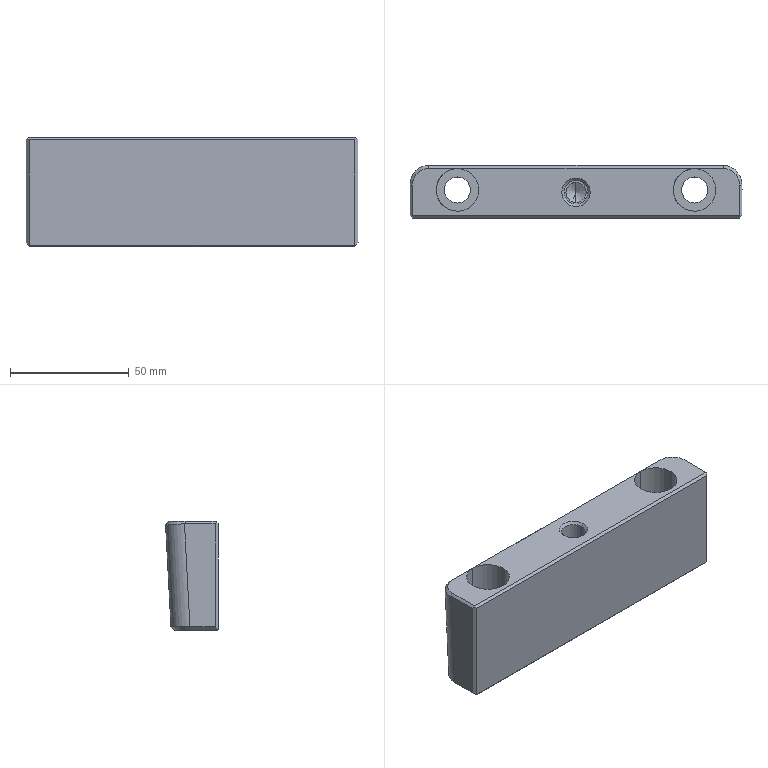Part | Creo | 1 solid | 41 faces | box 140 x 22.308 x 46 mm | volume 119302 mm3 | plane 19 | cylinder 14 | cone 4 | spline 4 | commonest cylinder face diameters 11 x4 18 x4 8.5 x2 10 x2 16 x2
STEP:
#1=CARTESIAN_POINT('',(-4.75,220.995,-77.8));
#2=VERTEX_POINT('',#1);
#3=CARTESIAN_POINT('',(5.25,220.995,-77.8));
#4=VERTEX_POINT('',#3);
#5=CARTESIAN_POINT('',(0.25,220.995,-77.8));
#6=DIRECTION('',(0.,0.,1.));
#7=DIRECTION('',(-1.,0.,0.));
#8=AXIS2_PLACEMENT_3D('',#5,#6,#7);
#9=CIRCLE('',#8,5.);
#10=EDGE_CURVE('',#2,#4,#9,.T.);
#11=ORIENTED_EDGE('',*,*,#10,.F.);
#12=CARTESIAN_POINT('',(0.25,220.995,-77.8));
#13=DIRECTION('',(0.,0.,1.));
#14=DIRECTION('',(1.,0.,0.));
#15=AXIS2_PLACEMENT_3D('',#12,#13,#14);
#16=CIRCLE('',#15,5.);
#17=EDGE_CURVE('',#4,#2,#16,.T.);
#18=ORIENTED_EDGE('',*,*,#17,.F.);
#19=EDGE_LOOP('',(#11,#18));
#20=FACE_OUTER_BOUND('',#19,.F.);
#21=CARTESIAN_POINT('',(-4.,220.995,-77.8));
#22=VERTEX_POINT('',#21);
#23=CARTESIAN_POINT('',(0.25,225.245,-77.8));
#24=VERTEX_POINT('',#23);
#25=CARTESIAN_POINT('',(0.25,220.995,-77.8));
#26=DIRECTION('',(0.,0.,-1.));
#27=DIRECTION('',(-1.,0.,0.));
#28=AXIS2_PLACEMENT_3D('',#25,#26,#27);
#29=CIRCLE('',#28,4.25);
#30=EDGE_CURVE('',#22,#24,#29,.T.);
#31=ORIENTED_EDGE('',*,*,#30,.F.);
#32=CARTESIAN_POINT('',(0.25,216.745,-77.8));
#33=VERTEX_POINT('',#32);
#34=CARTESIAN_POINT('',(0.25,220.995,-77.8));
#35=DIRECTION('',(0.,0.,-1.));
#36=DIRECTION('',(0.000000059,-1.,0.));
#37=AXIS2_PLACEMENT_3D('',#34,#35,#36);
#38=CIRCLE('',#37,4.25);
#39=EDGE_CURVE('',#33,#22,#38,.T.);
#40=ORIENTED_EDGE('',*,*,#39,.F.);
#41=CARTESIAN_POINT('',(0.25,220.995,-77.8));
#42=DIRECTION('',(0.,0.,-1.));
#43=DIRECTION('',(-0.000000059,1.,0.));
#44=AXIS2_PLACEMENT_3D('',#41,#42,#43);
#45=CIRCLE('',#44,4.25);
#46=EDGE_CURVE('',#24,#33,#45,.T.);
#47=ORIENTED_EDGE('',*,*,#46,.F.);
#48=EDGE_LOOP('',(#31,#40,#47));
#49=FACE_BOUND('',#48,.F.);
#50=CARTESIAN_POINT('',(0.25,220.995,-77.8));
#51=DIRECTION('',(0.,0.,-1.));
#52=DIRECTION('',(-1.,0.,0.));
#53=AXIS2_PLACEMENT_3D('',#50,#51,#52);
#54=PLANE('',#53);
#55=ADVANCED_FACE('',(#20,#49),#54,.F.);
#56=ORIENTED_EDGE('',*,*,#39,.T.);
#57=ORIENTED_EDGE('',*,*,#30,.T.);
#58=CARTESIAN_POINT('',(0.25,225.245,-86.8));
#59=VERTEX_POINT('',#58);
#60=CARTESIAN_POINT('',(0.25,225.245,-86.8));
#61=DIRECTION('',(0.,0.,1.));
#62=VECTOR('',#61,9.);
#63=LINE('',#60,#62);
#64=EDGE_CURVE('',#59,#24,#63,.T.);
#65=ORIENTED_EDGE('',*,*,#64,.F.);
#66=CARTESIAN_POINT('',(0.25,216.745,-86.8));
#67=VERTEX_POINT('',#66);
#68=CARTESIAN_POINT('',(0.25,220.995,-86.8));
#69=DIRECTION('',(0.,0.,1.));
#70=DIRECTION('',(-0.000000059,1.,0.));
#71=AXIS2_PLACEMENT_3D('',#68,#69,#70);
#72=CIRCLE('',#71,4.25);
#73=EDGE_CURVE('',#59,#67,#72,.T.);
#74=ORIENTED_EDGE('',*,*,#73,.T.);
#75=CARTESIAN_POINT('',(0.25,216.745,-86.8));
#76=DIRECTION('',(0.,0.,1.));
#77=VECTOR('',#76,9.);
#78=LINE('',#75,#77);
#79=EDGE_CURVE('',#67,#33,#78,.T.);
#80=ORIENTED_EDGE('',*,*,#79,.T.);
#81=EDGE_LOOP('',(#56,#57,#65,#74,#80));
#82=FACE_OUTER_BOUND('',#81,.F.);
#83=CARTESIAN_POINT('',(0.25,220.995,-90.756));
#84=DIRECTION('',(0.,0.,1.));
#85=DIRECTION('',(-0.000000059,1.,0.));
#86=AXIS2_PLACEMENT_3D('',#83,#84,#85);
#87=CYLINDRICAL_SURFACE('',#86,4.25);
#88=ADVANCED_FACE('',(#82),#87,.F.);
#89=ORIENTED_EDGE('',*,*,#46,.T.);
#90=ORIENTED_EDGE('',*,*,#79,.F.);
#91=CARTESIAN_POINT('',(0.25,220.995,-86.8));
#92=DIRECTION('',(0.,0.,1.));
#93=DIRECTION('',(0.000000059,-1.,0.));
#94=AXIS2_PLACEMENT_3D('',#91,#92,#93);
#95=CIRCLE('',#94,4.25);
#96=EDGE_CURVE('',#67,#59,#95,.T.);
#97=ORIENTED_EDGE('',*,*,#96,.T.);
#98=ORIENTED_EDGE('',*,*,#64,.T.);
#99=EDGE_LOOP('',(#89,#90,#97,#98));
#100=FACE_OUTER_BOUND('',#99,.F.);
#101=CARTESIAN_POINT('',(0.25,220.995,-90.756));
#102=DIRECTION('',(0.,0.,1.));
#103=DIRECTION('',(-0.000000059,1.,0.));
#104=AXIS2_PLACEMENT_3D('',#101,#102,#103);
#105=CYLINDRICAL_SURFACE('',#104,4.25);
#106=ADVANCED_FACE('',(#100),#105,.F.);
#107=ORIENTED_EDGE('',*,*,#96,.F.);
#108=CARTESIAN_POINT('',(0.25,220.995,-89.354));
#109=VERTEX_POINT('',#108);
#110=CARTESIAN_POINT('',(0.25,220.995,-89.354));
#111=DIRECTION('',(0.00000005,-0.8572,0.515));
#112=VECTOR('',#111,4.958);
#113=LINE('',#110,#112);
#114=EDGE_CURVE('',#109,#67,#113,.T.);
#115=ORIENTED_EDGE('',*,*,#114,.F.);
#116=CARTESIAN_POINT('',(0.25,220.995,-89.354));
#117=DIRECTION('',(-0.00000005,0.8572,0.515));
#118=VECTOR('',#117,4.958);
#119=LINE('',#116,#118);
#120=EDGE_CURVE('',#109,#59,#119,.T.);
#121=ORIENTED_EDGE('',*,*,#120,.T.);
#122=EDGE_LOOP('',(#107,#115,#121));
#123=FACE_OUTER_BOUND('',#122,.F.);
#124=CARTESIAN_POINT('',(0.25,220.995,-88.03));
#125=DIRECTION('',(0.,0.,1.));
#126=DIRECTION('',(-0.000000059,1.,0.));
#127=AXIS2_PLACEMENT_3D('',#124,#125,#126);
#128=CONICAL_SURFACE('',#127,2.202,59.);
#129=ADVANCED_FACE('',(#123),#128,.F.);
#130=ORIENTED_EDGE('',*,*,#73,.F.);
#131=ORIENTED_EDGE('',*,*,#120,.F.);
#132=ORIENTED_EDGE('',*,*,#114,.T.);
#133=EDGE_LOOP('',(#130,#131,#132));
#134=FACE_OUTER_BOUND('',#133,.F.);
#135=CARTESIAN_POINT('',(0.25,220.995,-88.03));
#136=DIRECTION('',(0.,0.,1.));
#137=DIRECTION('',(-0.000000059,1.,0.));
#138=AXIS2_PLACEMENT_3D('',#135,#136,#137);
#139=CONICAL_SURFACE('',#138,2.202,59.);
#140=ADVANCED_FACE('',(#134),#139,.F.);
#141=CARTESIAN_POINT('',(5.25,220.995,-55.));
#142=VERTEX_POINT('',#141);
#143=CARTESIAN_POINT('',(-4.75,220.995,-55.));
#144=VERTEX_POINT('',#143);
#145=CARTESIAN_POINT('',(0.25,220.995,-55.));
#146=DIRECTION('',(0.,0.,-1.));
#147=DIRECTION('',(1.,0.,0.));
#148=AXIS2_PLACEMENT_3D('',#145,#146,#147);
#149=CIRCLE('',#148,5.);
#150=EDGE_CURVE('',#142,#144,#149,.T.);
#151=ORIENTED_EDGE('',*,*,#150,.T.);
#152=CARTESIAN_POINT('',(-4.75,220.995,-55.));
#153=DIRECTION('',(0.,0.,-1.));
#154=VECTOR('',#153,22.8);
#155=LINE('',#152,#154);
#156=EDGE_CURVE('',#144,#2,#155,.T.);
#157=ORIENTED_EDGE('',*,*,#156,.T.);
#158=ORIENTED_EDGE('',*,*,#10,.T.);
#159=CARTESIAN_POINT('',(5.25,220.995,-55.));
#160=DIRECTION('',(0.,0.,-1.));
#161=VECTOR('',#160,22.8);
#162=LINE('',#159,#161);
#163=EDGE_CURVE('',#142,#4,#162,.T.);
#164=ORIENTED_EDGE('',*,*,#163,.F.);
#165=EDGE_LOOP('',(#151,#157,#158,#164));
#166=FACE_OUTER_BOUND('',#165,.F.);
#167=CARTESIAN_POINT('',(0.25,220.995,-50.3));
#168=DIRECTION('',(0.,0.,-1.));
#169=DIRECTION('',(-1.,0.,0.));
#170=AXIS2_PLACEMENT_3D('',#167,#168,#169);
#171=CYLINDRICAL_SURFACE('',#170,5.);
#172=ADVANCED_FACE('',(#166),#171,.F.);
#173=CARTESIAN_POINT('',(6.25,220.995,-54.));
#174=VERTEX_POINT('',#173);
#175=CARTESIAN_POINT('',(-5.75,220.995,-54.));
#176=VERTEX_POINT('',#175);
#177=CARTESIAN_POINT('',(0.25,220.995,-54.));
#178=DIRECTION('',(0.,0.,-1.));
#179=DIRECTION('',(1.,0.,0.));
#180=AXIS2_PLACEMENT_3D('',#177,#178,#179);
#181=CIRCLE('',#180,6.);
#182=EDGE_CURVE('',#174,#176,#181,.T.);
#183=ORIENTED_EDGE('',*,*,#182,.T.);
#184=CARTESIAN_POINT('',(-4.75,220.995,-55.));
#185=DIRECTION('',(-0.7071,0.,0.7071));
#186=VECTOR('',#185,1.414);
#187=LINE('',#184,#186);
#188=EDGE_CURVE('',#144,#176,#187,.T.);
#189=ORIENTED_EDGE('',*,*,#188,.F.);
#190=ORIENTED_EDGE('',*,*,#150,.F.);
#191=CARTESIAN_POINT('',(5.25,220.995,-55.));
#192=DIRECTION('',(0.7071,0.,0.7071));
#193=VECTOR('',#192,1.414);
#194=LINE('',#191,#193);
#195=EDGE_CURVE('',#142,#174,#194,.T.);
#196=ORIENTED_EDGE('',*,*,#195,.T.);
#197=EDGE_LOOP('',(#183,#189,#190,#196));
#198=FACE_OUTER_BOUND('',#197,.F.);
#199=CARTESIAN_POINT('',(0.25,220.995,-54.5));
#200=DIRECTION('',(0.,0.,1.));
#201=DIRECTION('',(1.,0.,0.));
#202=AXIS2_PLACEMENT_3D('',#199,#200,#201);
#203=CONICAL_SURFACE('',#202,5.5,45.);
#204=ADVANCED_FACE('',(#198),#203,.F.);
#205=CARTESIAN_POINT('',(-68.75,210.995,-54.));
#206=VERTEX_POINT('',#205);
#207=CARTESIAN_POINT('',(-68.75,224.025,-54.));
#208=VERTEX_POINT('',#207);
#209=CARTESIAN_POINT('',(-68.75,210.995,-54.));
#210=DIRECTION('',(0.000008474,1.,0.));
#211=VECTOR('',#210,13.03);
#212=LINE('',#209,#211);
#213=EDGE_CURVE('',#206,#208,#212,.T.);
#214=ORIENTED_EDGE('',*,*,#213,.T.);
#215=CARTESIAN_POINT('',(-61.751,231.036,-54.));
#216=VERTEX_POINT('',#215);
#217=CARTESIAN_POINT('',(-61.745,224.031,-54.));
#218=DIRECTION('',(0.,0.,1.));
#219=DIRECTION('',(-0.001152,1.,0.));
#220=AXIS2_PLACEMENT_3D('',#217,#218,#219);
#221=CIRCLE('',#220,7.005);
#222=EDGE_CURVE('',#216,#208,#221,.T.);
#223=ORIENTED_EDGE('',*,*,#222,.F.);
#224=CARTESIAN_POINT('',(62.253,231.036,-54.));
#225=VERTEX_POINT('',#224);
#226=CARTESIAN_POINT('',(-61.751,231.036,-54.));
#227=DIRECTION('',(1.,0.000000059,0.));
#228=VECTOR('',#227,124.002);
#229=LINE('',#226,#228);
#230=EDGE_CURVE('',#216,#225,#229,.T.);
#231=ORIENTED_EDGE('',*,*,#230,.T.);
#232=CARTESIAN_POINT('',(69.25,224.025,-54.));
#233=VERTEX_POINT('',#232);
#234=CARTESIAN_POINT('',(62.245,224.031,-54.));
#235=DIRECTION('',(0.,0.,1.));
#236=DIRECTION('',(1.,-0.001156,0.));
#237=AXIS2_PLACEMENT_3D('',#234,#235,#236);
#238=CIRCLE('',#237,7.005);
#239=EDGE_CURVE('',#233,#225,#238,.T.);
#240=ORIENTED_EDGE('',*,*,#239,.F.);
#241=CARTESIAN_POINT('',(69.25,210.995,-54.));
#242=VERTEX_POINT('',#241);
#243=CARTESIAN_POINT('',(69.25,224.025,-54.));
#244=DIRECTION('',(0.000004325,-1.,0.000004267));
#245=VECTOR('',#244,13.03);
#246=LINE('',#243,#245);
#247=EDGE_CURVE('',#233,#242,#246,.T.);
#248=ORIENTED_EDGE('',*,*,#247,.T.);
#249=CARTESIAN_POINT('',(69.25,210.995,-54.));
#250=DIRECTION('',(-1.,-0.000000059,0.));
#251=VECTOR('',#250,138.);
#252=LINE('',#249,#251);
#253=EDGE_CURVE('',#242,#206,#252,.T.);
#254=ORIENTED_EDGE('',*,*,#253,.T.);
#255=EDGE_LOOP('',(#214,#223,#231,#240,#248,#254));
#256=FACE_OUTER_BOUND('',#255,.F.);
#257=CARTESIAN_POINT('',(0.25,220.995,-54.));
#258=DIRECTION('',(0.,0.,-1.));
#259=DIRECTION('',(-1.,0.,0.));
#260=AXIS2_PLACEMENT_3D('',#257,#258,#259);
#261=CIRCLE('',#260,6.);
#262=EDGE_CURVE('',#176,#174,#261,.T.);
#263=ORIENTED_EDGE('',*,*,#262,.F.);
#264=ORIENTED_EDGE('',*,*,#182,.F.);
#265=EDGE_LOOP('',(#263,#264));
#266=FACE_BOUND('',#265,.F.);
#267=CARTESIAN_POINT('',(41.25,221.995,-54.));
#268=VERTEX_POINT('',#267);
#269=CARTESIAN_POINT('',(50.25,230.995,-54.));
#270=VERTEX_POINT('',#269);
#271=CARTESIAN_POINT('',(50.25,221.995,-54.));
#272=DIRECTION('',(0.,0.,-1.));
#273=DIRECTION('',(-1.,0.,0.));
#274=AXIS2_PLACEMENT_3D('',#271,#272,#273);
#275=CIRCLE('',#274,9.);
#276=EDGE_CURVE('',#268,#270,#275,.T.);
#277=ORIENTED_EDGE('',*,*,#276,.F.);
#278=CARTESIAN_POINT('',(50.25,212.995,-54.));
#279=VERTEX_POINT('',#278);
#280=CARTESIAN_POINT('',(50.25,221.995,-54.));
#281=DIRECTION('',(0.,0.,-1.));
#282=DIRECTION('',(0.000000059,-1.,0.));
#283=AXIS2_PLACEMENT_3D('',#280,#281,#282);
#284=CIRCLE('',#283,9.);
#285=EDGE_CURVE('',#279,#268,#284,.T.);
#286=ORIENTED_EDGE('',*,*,#285,.F.);
#287=CARTESIAN_POINT('',(50.25,221.995,-54.));
#288=DIRECTION('',(0.,0.,-1.));
#289=DIRECTION('',(-0.000000059,1.,0.));
#290=AXIS2_PLACEMENT_3D('',#287,#288,#289);
#291=CIRCLE('',#290,9.);
#292=EDGE_CURVE('',#270,#279,#291,.T.);
#293=ORIENTED_EDGE('',*,*,#292,.F.);
#294=EDGE_LOOP('',(#277,#286,#293));
#295=FACE_BOUND('',#294,.F.);
#296=CARTESIAN_POINT('',(-58.75,221.995,-54.));
#297=VERTEX_POINT('',#296);
#298=CARTESIAN_POINT('',(-49.75,230.995,-54.));
#299=VERTEX_POINT('',#298);
#300=CARTESIAN_POINT('',(-49.75,221.995,-54.));
#301=DIRECTION('',(0.,0.,-1.));
#302=DIRECTION('',(-1.,0.,0.));
#303=AXIS2_PLACEMENT_3D('',#300,#301,#302);
#304=CIRCLE('',#303,9.);
#305=EDGE_CURVE('',#297,#299,#304,.T.);
#306=ORIENTED_EDGE('',*,*,#305,.F.);
#307=CARTESIAN_POINT('',(-49.75,212.995,-54.));
#308=VERTEX_POINT('',#307);
#309=CARTESIAN_POINT('',(-49.75,221.995,-54.));
#310=DIRECTION('',(0.,0.,-1.));
#311=DIRECTION('',(0.000000059,-1.,0.));
#312=AXIS2_PLACEMENT_3D('',#309,#310,#311);
#313=CIRCLE('',#312,9.);
#314=EDGE_CURVE('',#308,#297,#313,.T.);
#315=ORIENTED_EDGE('',*,*,#314,.F.);
#316=CARTESIAN_POINT('',(-49.75,221.995,-54.));
#317=DIRECTION('',(0.,0.,-1.));
#318=DIRECTION('',(-0.000000059,1.,0.));
#319=AXIS2_PLACEMENT_3D('',#316,#317,#318);
#320=CIRCLE('',#319,9.);
#321=EDGE_CURVE('',#299,#308,#320,.T.);
#322=ORIENTED_EDGE('',*,*,#321,.F.);
#323=EDGE_LOOP('',(#306,#315,#322));
#324=FACE_BOUND('',#323,.F.);
#325=CARTESIAN_POINT('',(0.25,286.495,-54.));
#326=DIRECTION('',(0.,0.,-1.));
#327=DIRECTION('',(-1.,0.,0.));
#328=AXIS2_PLACEMENT_3D('',#325,#326,#327);
#329=PLANE('',#328);
#330=ADVANCED_FACE('',(#256,#266,#295,#324),#329,.F.);
#331=CARTESIAN_POINT('',(-69.75,224.026,-55.));
#332=VERTEX_POINT('',#331);
#333=CARTESIAN_POINT('',(-69.75,211.419,-55.));
#334=VERTEX_POINT('',#333);
#335=CARTESIAN_POINT('',(-69.75,224.026,-55.));
#336=DIRECTION('',(-0.000003827,-1.,0.000003886));
#337=VECTOR('',#336,12.608);
#338=LINE('',#335,#337);
#339=EDGE_CURVE('',#332,#334,#338,.T.);
#340=ORIENTED_EDGE('',*,*,#339,.F.);
#341=CARTESIAN_POINT('',(-69.75,224.026,-55.));
#342=DIRECTION('',(0.7071,-0.0006986,0.7071));
#343=VECTOR('',#342,1.414);
#344=LINE('',#341,#343);
#345=EDGE_CURVE('',#332,#208,#344,.T.);
#346=ORIENTED_EDGE('',*,*,#345,.T.);
#347=ORIENTED_EDGE('',*,*,#213,.F.);
#348=CARTESIAN_POINT('',(-69.038,210.707,-54.288));
#349=VERTEX_POINT('',#348);
#350=CARTESIAN_POINT('',(-69.038,210.707,-54.288));
#351=DIRECTION('',(0.5774,0.5774,0.5774));
#352=VECTOR('',#351,0.4993);
#353=LINE('',#350,#352);
#354=EDGE_CURVE('',#349,#206,#353,.T.);
#355=ORIENTED_EDGE('',*,*,#354,.F.);
#356=CARTESIAN_POINT('',(-69.75,211.419,-55.));
#357=DIRECTION('',(0.5774,-0.5774,0.5774));
#358=VECTOR('',#357,1.233);
#359=LINE('',#356,#358);
#360=EDGE_CURVE('',#334,#349,#359,.T.);
#361=ORIENTED_EDGE('',*,*,#360,.F.);
#362=EDGE_LOOP('',(#340,#346,#347,#355,#361));
#363=FACE_OUTER_BOUND('',#362,.F.);
#364=CARTESIAN_POINT('',(-69.75,209.995,-55.));
#365=DIRECTION('',(0.7071,0.000000042,-0.7071));
#366=DIRECTION('',(-0.000000059,1.,0.));
#367=AXIS2_PLACEMENT_3D('',#364,#365,#366);
#368=PLANE('',#367);
#369=ADVANCED_FACE('',(#363),#368,.F.);
#370=CARTESIAN_POINT('',(-69.75,211.419,-98.419));
#371=VERTEX_POINT('',#370);
#372=CARTESIAN_POINT('',(-69.75,211.419,-55.));
#373=DIRECTION('',(0.,0.,-1.));
#374=VECTOR('',#373,43.419);
#375=LINE('',#372,#374);
#376=EDGE_CURVE('',#334,#371,#375,.T.);
#377=ORIENTED_EDGE('',*,*,#376,.T.);
#378=CARTESIAN_POINT('',(-69.75,222.039,-98.419));
#379=VERTEX_POINT('',#378);
#380=CARTESIAN_POINT('',(-69.75,211.419,-98.419));
#381=DIRECTION('',(-0.000000059,1.,-0.00001364));
#382=VECTOR('',#381,10.62);
#383=LINE('',#380,#382);
#384=EDGE_CURVE('',#371,#379,#383,.T.);
#385=ORIENTED_EDGE('',*,*,#384,.T.);
#386=CARTESIAN_POINT('',(-69.75,224.314,-55.007));
#387=VERTEX_POINT('',#386);
#388=CARTESIAN_POINT('',(-69.75,224.314,-55.007));
#389=DIRECTION('',(-0.000000814,-0.05234,-0.9986));
#390=VECTOR('',#389,43.472);
#391=LINE('',#388,#390);
#392=EDGE_CURVE('',#387,#379,#391,.T.);
#393=ORIENTED_EDGE('',*,*,#392,.F.);
#394=CARTESIAN_POINT('',(-69.75,224.026,-55.));
#395=CARTESIAN_POINT('',(-69.75,224.058,-55.));
#396=CARTESIAN_POINT('',(-69.75,224.122,-55.001));
#397=CARTESIAN_POINT('',(-69.75,224.218,-55.003));
#398=CARTESIAN_POINT('',(-69.75,224.282,-55.006));
#399=B_SPLINE_CURVE_WITH_KNOTS('',3,(#394,#395,#396,#397,#398,#386),.UNSPECIFIED.,.F.,.F.,(4,1,1,4),(0.,0.3333,0.6667,1.),.UNSPECIFIED.);
#400=EDGE_CURVE('',#332,#387,#399,.T.);
#401=ORIENTED_EDGE('',*,*,#400,.F.);
#402=ORIENTED_EDGE('',*,*,#339,.T.);
#403=EDGE_LOOP('',(#377,#385,#393,#401,#402));
#404=FACE_OUTER_BOUND('',#403,.F.);
#405=CARTESIAN_POINT('',(-69.75,209.995,-61.3));
#406=DIRECTION('',(1.,0.000000059,0.));
#407=DIRECTION('',(-0.000000059,1.,0.));
#408=AXIS2_PLACEMENT_3D('',#405,#406,#407);
#409=PLANE('',#408);
#410=ADVANCED_FACE('',(#404),#409,.F.);
#411=CARTESIAN_POINT('',(-68.498,210.167,-99.671));
#412=VERTEX_POINT('',#411);
#413=CARTESIAN_POINT('',(-69.75,211.419,-98.419));
#414=DIRECTION('',(0.5774,-0.5774,-0.5774));
#415=VECTOR('',#414,2.169);
#416=LINE('',#413,#415);
#417=EDGE_CURVE('',#371,#412,#416,.T.);
#418=ORIENTED_EDGE('',*,*,#417,.F.);
#419=ORIENTED_EDGE('',*,*,#376,.F.);
#420=ORIENTED_EDGE('',*,*,#360,.T.);
#421=CARTESIAN_POINT('',(-68.331,210.,-54.995));
#422=VERTEX_POINT('',#421);
#423=CARTESIAN_POINT('',(-69.038,210.707,-54.288));
#424=DIRECTION('',(0.5774,-0.5774,-0.5774));
#425=VECTOR('',#424,1.225);
#426=LINE('',#423,#425);
#427=EDGE_CURVE('',#349,#422,#426,.T.);
#428=ORIENTED_EDGE('',*,*,#427,.T.);
#429=CARTESIAN_POINT('',(-68.331,210.,-99.505));
#430=VERTEX_POINT('',#429);
#431=CARTESIAN_POINT('',(-68.331,210.,-54.995));
#432=DIRECTION('',(0.,0.,-1.));
#433=VECTOR('',#432,44.509);
#434=LINE('',#431,#433);
#435=EDGE_CURVE('',#422,#430,#434,.T.);
#436=ORIENTED_EDGE('',*,*,#435,.T.);
#437=CARTESIAN_POINT('',(-68.331,210.,-99.505));
#438=DIRECTION('',(-0.5774,0.5774,-0.5774));
#439=VECTOR('',#438,0.2887);
#440=LINE('',#437,#439);
#441=EDGE_CURVE('',#430,#412,#440,.T.);
#442=ORIENTED_EDGE('',*,*,#441,.T.);
#443=EDGE_LOOP('',(#418,#419,#420,#428,#436,#442));
#444=FACE_OUTER_BOUND('',#443,.F.);
#445=CARTESIAN_POINT('',(-69.038,210.707,-79.86));
#446=DIRECTION('',(-0.7071,-0.7071,0.));
#447=DIRECTION('',(0.7071,-0.7071,0.));
#448=AXIS2_PLACEMENT_3D('',#445,#446,#447);
#449=PLANE('',#448);
#450=ADVANCED_FACE('',(#444),#449,.T.);
#451=CARTESIAN_POINT('',(-68.169,210.495,-100.));
#452=VERTEX_POINT('',#451);
#453=CARTESIAN_POINT('',(-68.169,222.04,-100.));
#454=VERTEX_POINT('',#453);
#455=CARTESIAN_POINT('',(-68.169,210.495,-100.));
#456=DIRECTION('',(-0.000003417,1.,-0.000003359));
#457=VECTOR('',#456,11.544);
#458=LINE('',#455,#457);
#459=EDGE_CURVE('',#452,#454,#458,.T.);
#460=ORIENTED_EDGE('',*,*,#459,.T.);
#461=CARTESIAN_POINT('',(-68.169,222.04,-100.));
#462=DIRECTION('',(-0.7071,-0.0003107,0.7071));
#463=VECTOR('',#462,2.235);
#464=LINE('',#461,#463);
#465=EDGE_CURVE('',#454,#379,#464,.T.);
#466=ORIENTED_EDGE('',*,*,#465,.T.);
#467=ORIENTED_EDGE('',*,*,#384,.F.);
#468=ORIENTED_EDGE('',*,*,#417,.T.);
#469=CARTESIAN_POINT('',(-68.498,210.167,-99.671));
#470=DIRECTION('',(0.5774,0.5774,-0.5774));
#471=VECTOR('',#470,0.5692);
#472=LINE('',#469,#471);
#473=EDGE_CURVE('',#412,#452,#472,.T.);
#474=ORIENTED_EDGE('',*,*,#473,.T.);
#475=EDGE_LOOP('',(#460,#466,#467,#468,#474));
#476=FACE_OUTER_BOUND('',#475,.F.);
#477=CARTESIAN_POINT('',(-68.96,216.017,-99.21));
#478=DIRECTION('',(-0.7071,-0.000000042,-0.7071));
#479=DIRECTION('',(0.7071,0.000000042,-0.7071));
#480=AXIS2_PLACEMENT_3D('',#477,#478,#479);
#481=PLANE('',#480);
#482=ADVANCED_FACE('',(#476),#481,.T.);
#483=CARTESIAN_POINT('',(68.669,222.04,-100.));
#484=VERTEX_POINT('',#483);
#485=CARTESIAN_POINT('',(68.669,210.495,-100.));
#486=VERTEX_POINT('',#485);
#487=CARTESIAN_POINT('',(68.669,222.04,-100.));
#488=DIRECTION('',(-0.0000033,-1.,0.000003359));
#489=VECTOR('',#488,11.544);
#490=LINE('',#487,#489);
#491=EDGE_CURVE('',#484,#486,#490,.T.);
#492=ORIENTED_EDGE('',*,*,#491,.F.);
#493=CARTESIAN_POINT('',(62.251,228.467,-100.));
#494=VERTEX_POINT('',#493);
#495=CARTESIAN_POINT('',(62.251,228.467,-100.));
#496=CARTESIAN_POINT('',(62.623,228.467,-100.));
#497=CARTESIAN_POINT('',(63.427,228.397,-100.));
#498=CARTESIAN_POINT('',(64.631,228.057,-100.));
#499=CARTESIAN_POINT('',(65.801,227.448,-100.));
#500=CARTESIAN_POINT('',(66.825,226.612,-100.));
#501=CARTESIAN_POINT('',(67.658,225.585,-100.));
#502=CARTESIAN_POINT('',(68.264,224.412,-100.));
#503=CARTESIAN_POINT('',(68.601,223.209,-100.));
#504=CARTESIAN_POINT('',(68.668,222.408,-100.));
#505=CARTESIAN_POINT('',(68.669,222.04,-100.));
#506=B_SPLINE_CURVE_WITH_KNOTS('',3,(#495,#496,#497,#498,#499,#500,#501,#502,#503,#504,#505),.UNSPECIFIED.,.F.,.F.,(4,1,1,1,1,1,1,1,4),(0.,0.112,0.2416,0.3712,0.5008,0.6304,0.76,0.8895,1.),.UNSPECIFIED.);
#507=EDGE_CURVE('',#494,#484,#506,.T.);
#508=ORIENTED_EDGE('',*,*,#507,.F.);
#509=CARTESIAN_POINT('',(-61.751,228.467,-100.));
#510=VERTEX_POINT('',#509);
#511=CARTESIAN_POINT('',(-61.751,228.467,-100.));
#512=DIRECTION('',(1.,0.000000059,0.));
#513=VECTOR('',#512,124.001);
#514=LINE('',#511,#513);
#515=EDGE_CURVE('',#510,#494,#514,.T.);
#516=ORIENTED_EDGE('',*,*,#515,.F.);
#517=CARTESIAN_POINT('',(-68.169,222.04,-100.));
#518=CARTESIAN_POINT('',(-68.17,222.408,-100.));
#519=CARTESIAN_POINT('',(-68.1,223.209,-100.));
#520=CARTESIAN_POINT('',(-67.764,224.412,-100.));
#521=CARTESIAN_POINT('',(-67.158,225.585,-100.));
#522=CARTESIAN_POINT('',(-66.325,226.612,-100.));
#523=CARTESIAN_POINT('',(-65.301,227.448,-100.));
#524=CARTESIAN_POINT('',(-64.131,228.056,-100.));
#525=CARTESIAN_POINT('',(-62.926,228.398,-100.));
#526=CARTESIAN_POINT('',(-62.123,228.466,-100.));
#527=CARTESIAN_POINT('',(-61.751,228.467,-100.));
#528=B_SPLINE_CURVE_WITH_KNOTS('',3,(#517,#518,#519,#520,#521,#522,#523,#524,#525,#526,#527),.UNSPECIFIED.,.F.,.F.,(4,1,1,1,1,1,1,1,4),(0.,0.1105,0.24,0.3696,0.4992,0.6288,0.7584,0.888,1.),.UNSPECIFIED.);
#529=EDGE_CURVE('',#454,#510,#528,.T.);
#530=ORIENTED_EDGE('',*,*,#529,.F.);
#531=ORIENTED_EDGE('',*,*,#459,.F.);
#532=CARTESIAN_POINT('',(-68.169,210.495,-100.));
#533=DIRECTION('',(1.,0.000000059,0.));
#534=VECTOR('',#533,136.839);
#535=LINE('',#532,#534);
#536=EDGE_CURVE('',#452,#486,#535,.T.);
#537=ORIENTED_EDGE('',*,*,#536,.T.);
#538=EDGE_LOOP('',(#492,#508,#516,#530,#531,#537));
#539=FACE_OUTER_BOUND('',#538,.F.);
#540=CARTESIAN_POINT('',(-49.75,227.495,-100.));
#541=VERTEX_POINT('',#540);
#542=CARTESIAN_POINT('',(-49.75,216.495,-100.));
#543=VERTEX_POINT('',#542);
#544=CARTESIAN_POINT('',(-49.75,221.995,-100.));
#545=DIRECTION('',(0.,0.,1.));
#546=DIRECTION('',(-0.000000059,1.,0.));
#547=AXIS2_PLACEMENT_3D('',#544,#545,#546);
#548=CIRCLE('',#547,5.5);
#549=EDGE_CURVE('',#541,#543,#548,.T.);
#550=ORIENTED_EDGE('',*,*,#549,.F.);
#551=CARTESIAN_POINT('',(-49.75,221.995,-100.));
#552=DIRECTION('',(0.,0.,1.));
#553=DIRECTION('',(0.000000059,-1.,0.));
#554=AXIS2_PLACEMENT_3D('',#551,#552,#553);
#555=CIRCLE('',#554,5.5);
#556=EDGE_CURVE('',#543,#541,#555,.T.);
#557=ORIENTED_EDGE('',*,*,#556,.F.);
#558=EDGE_LOOP('',(#550,#557));
#559=FACE_BOUND('',#558,.F.);
#560=CARTESIAN_POINT('',(50.25,227.495,-100.));
#561=VERTEX_POINT('',#560);
#562=CARTESIAN_POINT('',(50.25,216.495,-100.));
#563=VERTEX_POINT('',#562);
#564=CARTESIAN_POINT('',(50.25,221.995,-100.));
#565=DIRECTION('',(0.,0.,1.));
#566=DIRECTION('',(-0.000000059,1.,0.));
#567=AXIS2_PLACEMENT_3D('',#564,#565,#566);
#568=CIRCLE('',#567,5.5);
#569=EDGE_CURVE('',#561,#563,#568,.T.);
#570=ORIENTED_EDGE('',*,*,#569,.F.);
#571=CARTESIAN_POINT('',(50.25,221.995,-100.));
#572=DIRECTION('',(0.,0.,1.));
#573=DIRECTION('',(0.000000059,-1.,0.));
#574=AXIS2_PLACEMENT_3D('',#571,#572,#573);
#575=CIRCLE('',#574,5.5);
#576=EDGE_CURVE('',#563,#561,#575,.T.);
#577=ORIENTED_EDGE('',*,*,#576,.F.);
#578=EDGE_LOOP('',(#570,#577));
#579=FACE_BOUND('',#578,.F.);
#580=CARTESIAN_POINT('',(-69.75,209.995,-100.));
#581=DIRECTION('',(0.,0.,-1.));
#582=DIRECTION('',(-0.000000059,1.,0.));
#583=AXIS2_PLACEMENT_3D('',#580,#581,#582);
#584=PLANE('',#583);
#585=ADVANCED_FACE('',(#539,#559,#579),#584,.T.);
#586=ORIENTED_EDGE('',*,*,#569,.T.);
#587=CARTESIAN_POINT('',(50.25,216.495,-66.8));
#588=VERTEX_POINT('',#587);
#589=CARTESIAN_POINT('',(50.25,216.495,-100.));
#590=DIRECTION('',(0.,0.,1.));
#591=VECTOR('',#590,33.2);
#592=LINE('',#589,#591);
#593=EDGE_CURVE('',#563,#588,#592,.T.);
#594=ORIENTED_EDGE('',*,*,#593,.T.);
#595=CARTESIAN_POINT('',(50.25,227.495,-66.8));
#596=VERTEX_POINT('',#595);
#597=CARTESIAN_POINT('',(50.25,221.995,-66.8));
#598=DIRECTION('',(0.,0.,-1.));
#599=DIRECTION('',(0.000000059,-1.,0.));
#600=AXIS2_PLACEMENT_3D('',#597,#598,#599);
#601=CIRCLE('',#600,5.5);
#602=EDGE_CURVE('',#588,#596,#601,.T.);
#603=ORIENTED_EDGE('',*,*,#602,.T.);
#604=CARTESIAN_POINT('',(50.25,227.495,-100.));
#605=DIRECTION('',(0.,0.,1.));
#606=VECTOR('',#605,33.2);
#607=LINE('',#604,#606);
#608=EDGE_CURVE('',#561,#596,#607,.T.);
#609=ORIENTED_EDGE('',*,*,#608,.F.);
#610=EDGE_LOOP('',(#586,#594,#603,#609));
#611=FACE_OUTER_BOUND('',#610,.F.);
#612=CARTESIAN_POINT('',(50.25,221.995,-72.3));
#613=DIRECTION('',(0.,0.,1.));
#614=DIRECTION('',(-0.000000059,1.,0.));
#615=AXIS2_PLACEMENT_3D('',#612,#613,#614);
#616=CYLINDRICAL_SURFACE('',#615,5.5);
#617=ADVANCED_FACE('',(#611),#616,.F.);
#618=ORIENTED_EDGE('',*,*,#576,.T.);
#619=ORIENTED_EDGE('',*,*,#608,.T.);
#620=CARTESIAN_POINT('',(50.25,221.995,-66.8));
#621=DIRECTION('',(0.,0.,-1.));
#622=DIRECTION('',(-0.000000059,1.,0.));
#623=AXIS2_PLACEMENT_3D('',#620,#621,#622);
#624=CIRCLE('',#623,5.5);
#625=EDGE_CURVE('',#596,#588,#624,.T.);
#626=ORIENTED_EDGE('',*,*,#625,.T.);
#627=ORIENTED_EDGE('',*,*,#593,.F.);
#628=EDGE_LOOP('',(#618,#619,#626,#627));
#629=FACE_OUTER_BOUND('',#628,.F.);
#630=CARTESIAN_POINT('',(50.25,221.995,-72.3));
#631=DIRECTION('',(0.,0.,1.));
#632=DIRECTION('',(-0.000000059,1.,0.));
#633=AXIS2_PLACEMENT_3D('',#630,#631,#632);
#634=CYLINDRICAL_SURFACE('',#633,5.5);
#635=ADVANCED_FACE('',(#629),#634,.F.);
#636=CARTESIAN_POINT('',(50.25,230.995,-66.8));
#637=VERTEX_POINT('',#636);
#638=CARTESIAN_POINT('',(50.25,212.995,-66.8));
#639=VERTEX_POINT('',#638);
#640=CARTESIAN_POINT('',(50.25,221.995,-66.8));
#641=DIRECTION('',(0.,0.,1.));
#642=DIRECTION('',(-0.000000059,1.,0.));
#643=AXIS2_PLACEMENT_3D('',#640,#641,#642);
#644=CIRCLE('',#643,9.);
#645=EDGE_CURVE('',#637,#639,#644,.T.);
#646=ORIENTED_EDGE('',*,*,#645,.F.);
#647=CARTESIAN_POINT('',(50.25,221.995,-66.8));
#648=DIRECTION('',(0.,0.,1.));
#649=DIRECTION('',(0.000000059,-1.,0.));
#650=AXIS2_PLACEMENT_3D('',#647,#648,#649);
#651=CIRCLE('',#650,9.);
#652=EDGE_CURVE('',#639,#637,#651,.T.);
#653=ORIENTED_EDGE('',*,*,#652,.F.);
#654=EDGE_LOOP('',(#646,#653));
#655=FACE_OUTER_BOUND('',#654,.F.);
#656=ORIENTED_EDGE('',*,*,#625,.F.);
#657=ORIENTED_EDGE('',*,*,#602,.F.);
#658=EDGE_LOOP('',(#656,#657));
#659=FACE_BOUND('',#658,.F.);
#660=CARTESIAN_POINT('',(50.25,221.995,-66.8));
#661=DIRECTION('',(0.,0.,-1.));
#662=DIRECTION('',(-0.000000059,1.,0.));
#663=AXIS2_PLACEMENT_3D('',#660,#661,#662);
#664=PLANE('',#663);
#665=ADVANCED_FACE('',(#655,#659),#664,.F.);
#666=ORIENTED_EDGE('',*,*,#285,.T.);
#667=ORIENTED_EDGE('',*,*,#276,.T.);
#668=CARTESIAN_POINT('',(50.25,230.995,-54.));
#669=DIRECTION('',(0.,0.,-1.));
#670=VECTOR('',#669,12.8);
#671=LINE('',#668,#670);
#672=EDGE_CURVE('',#270,#637,#671,.T.);
#673=ORIENTED_EDGE('',*,*,#672,.T.);
#674=ORIENTED_EDGE('',*,*,#645,.T.);
#675=CARTESIAN_POINT('',(50.25,212.995,-54.));
#676=DIRECTION('',(0.,0.,-1.));
#677=VECTOR('',#676,12.8);
#678=LINE('',#675,#677);
#679=EDGE_CURVE('',#279,#639,#678,.T.);
#680=ORIENTED_EDGE('',*,*,#679,.F.);
#681=EDGE_LOOP('',(#666,#667,#673,#674,#680));
#682=FACE_OUTER_BOUND('',#681,.F.);
#683=CARTESIAN_POINT('',(50.25,221.995,-55.25));
#684=DIRECTION('',(0.,0.,-1.));
#685=DIRECTION('',(-0.000000059,1.,0.));
#686=AXIS2_PLACEMENT_3D('',#683,#684,#685);
#687=CYLINDRICAL_SURFACE('',#686,9.);
#688=ADVANCED_FACE('',(#682),#687,.F.);
#689=ORIENTED_EDGE('',*,*,#292,.T.);
#690=ORIENTED_EDGE('',*,*,#679,.T.);
#691=ORIENTED_EDGE('',*,*,#652,.T.);
#692=ORIENTED_EDGE('',*,*,#672,.F.);
#693=EDGE_LOOP('',(#689,#690,#691,#692));
#694=FACE_OUTER_BOUND('',#693,.F.);
#695=CARTESIAN_POINT('',(50.25,221.995,-55.25));
#696=DIRECTION('',(0.,0.,-1.));
#697=DIRECTION('',(-0.000000059,1.,0.));
#698=AXIS2_PLACEMENT_3D('',#695,#696,#697);
#699=CYLINDRICAL_SURFACE('',#698,9.);
#700=ADVANCED_FACE('',(#694),#699,.F.);
#701=ORIENTED_EDGE('',*,*,#549,.T.);
#702=CARTESIAN_POINT('',(-49.75,216.495,-66.8));
#703=VERTEX_POINT('',#702);
#704=CARTESIAN_POINT('',(-49.75,216.495,-100.));
#705=DIRECTION('',(0.,0.,1.));
#706=VECTOR('',#705,33.2);
#707=LINE('',#704,#706);
#708=EDGE_CURVE('',#543,#703,#707,.T.);
#709=ORIENTED_EDGE('',*,*,#708,.T.);
#710=CARTESIAN_POINT('',(-49.75,227.495,-66.8));
#711=VERTEX_POINT('',#710);
#712=CARTESIAN_POINT('',(-49.75,221.995,-66.8));
#713=DIRECTION('',(0.,0.,-1.));
#714=DIRECTION('',(0.000000059,-1.,0.));
#715=AXIS2_PLACEMENT_3D('',#712,#713,#714);
#716=CIRCLE('',#715,5.5);
#717=EDGE_CURVE('',#703,#711,#716,.T.);
#718=ORIENTED_EDGE('',*,*,#717,.T.);
#719=CARTESIAN_POINT('',(-49.75,227.495,-100.));
#720=DIRECTION('',(0.,0.,1.));
#721=VECTOR('',#720,33.2);
#722=LINE('',#719,#721);
#723=EDGE_CURVE('',#541,#711,#722,.T.);
#724=ORIENTED_EDGE('',*,*,#723,.F.);
#725=EDGE_LOOP('',(#701,#709,#718,#724));
#726=FACE_OUTER_BOUND('',#725,.F.);
#727=CARTESIAN_POINT('',(-49.75,221.995,-72.3));
#728=DIRECTION('',(0.,0.,1.));
#729=DIRECTION('',(-0.000000059,1.,0.));
#730=AXIS2_PLACEMENT_3D('',#727,#728,#729);
#731=CYLINDRICAL_SURFACE('',#730,5.5);
#732=ADVANCED_FACE('',(#726),#731,.F.);
#733=ORIENTED_EDGE('',*,*,#556,.T.);
#734=ORIENTED_EDGE('',*,*,#723,.T.);
#735=CARTESIAN_POINT('',(-49.75,221.995,-66.8));
#736=DIRECTION('',(0.,0.,-1.));
#737=DIRECTION('',(-0.000000059,1.,0.));
#738=AXIS2_PLACEMENT_3D('',#735,#736,#737);
#739=CIRCLE('',#738,5.5);
#740=EDGE_CURVE('',#711,#703,#739,.T.);
#741=ORIENTED_EDGE('',*,*,#740,.T.);
#742=ORIENTED_EDGE('',*,*,#708,.F.);
#743=EDGE_LOOP('',(#733,#734,#741,#742));
#744=FACE_OUTER_BOUND('',#743,.F.);
#745=CARTESIAN_POINT('',(-49.75,221.995,-72.3));
#746=DIRECTION('',(0.,0.,1.));
#747=DIRECTION('',(-0.000000059,1.,0.));
#748=AXIS2_PLACEMENT_3D('',#745,#746,#747);
#749=CYLINDRICAL_SURFACE('',#748,5.5);
#750=ADVANCED_FACE('',(#744),#749,.F.);
#751=CARTESIAN_POINT('',(-49.75,230.995,-66.8));
#752=VERTEX_POINT('',#751);
#753=CARTESIAN_POINT('',(-49.75,212.995,-66.8));
#754=VERTEX_POINT('',#753);
#755=CARTESIAN_POINT('',(-49.75,221.995,-66.8));
#756=DIRECTION('',(0.,0.,1.));
#757=DIRECTION('',(-0.000000059,1.,0.));
#758=AXIS2_PLACEMENT_3D('',#755,#756,#757);
#759=CIRCLE('',#758,9.);
#760=EDGE_CURVE('',#752,#754,#759,.T.);
#761=ORIENTED_EDGE('',*,*,#760,.F.);
#762=CARTESIAN_POINT('',(-49.75,221.995,-66.8));
#763=DIRECTION('',(0.,0.,1.));
#764=DIRECTION('',(0.000000059,-1.,0.));
#765=AXIS2_PLACEMENT_3D('',#762,#763,#764);
#766=CIRCLE('',#765,9.);
#767=EDGE_CURVE('',#754,#752,#766,.T.);
#768=ORIENTED_EDGE('',*,*,#767,.F.);
#769=EDGE_LOOP('',(#761,#768));
#770=FACE_OUTER_BOUND('',#769,.F.);
#771=ORIENTED_EDGE('',*,*,#740,.F.);
#772=ORIENTED_EDGE('',*,*,#717,.F.);
#773=EDGE_LOOP('',(#771,#772));
#774=FACE_BOUND('',#773,.F.);
#775=CARTESIAN_POINT('',(50.25,221.995,-66.8));
#776=DIRECTION('',(0.,0.,-1.));
#777=DIRECTION('',(-0.000000059,1.,0.));
#778=AXIS2_PLACEMENT_3D('',#775,#776,#777);
#779=PLANE('',#778);
#780=ADVANCED_FACE('',(#770,#774),#779,.F.);
#781=ORIENTED_EDGE('',*,*,#314,.T.);
#782=ORIENTED_EDGE('',*,*,#305,.T.);
#783=CARTESIAN_POINT('',(-49.75,230.995,-54.));
#784=DIRECTION('',(0.,0.,-1.));
#785=VECTOR('',#784,12.8);
#786=LINE('',#783,#785);
#787=EDGE_CURVE('',#299,#752,#786,.T.);
#788=ORIENTED_EDGE('',*,*,#787,.T.);
#789=ORIENTED_EDGE('',*,*,#760,.T.);
#790=CARTESIAN_POINT('',(-49.75,212.995,-54.));
#791=DIRECTION('',(0.,0.,-1.));
#792=VECTOR('',#791,12.8);
#793=LINE('',#790,#792);
#794=EDGE_CURVE('',#308,#754,#793,.T.);
#795=ORIENTED_EDGE('',*,*,#794,.F.);
#796=EDGE_LOOP('',(#781,#782,#788,#789,#795));
#797=FACE_OUTER_BOUND('',#796,.F.);
#798=CARTESIAN_POINT('',(-49.75,221.995,-55.25));
#799=DIRECTION('',(0.,0.,-1.));
#800=DIRECTION('',(-0.000000059,1.,0.));
#801=AXIS2_PLACEMENT_3D('',#798,#799,#800);
#802=CYLINDRICAL_SURFACE('',#801,9.);
#803=ADVANCED_FACE('',(#797),#802,.F.);
#804=ORIENTED_EDGE('',*,*,#321,.T.);
#805=ORIENTED_EDGE('',*,*,#794,.T.);
#806=ORIENTED_EDGE('',*,*,#767,.T.);
#807=ORIENTED_EDGE('',*,*,#787,.F.);
#808=EDGE_LOOP('',(#804,#805,#806,#807));
#809=FACE_OUTER_BOUND('',#808,.F.);
#810=CARTESIAN_POINT('',(-49.75,221.995,-55.25));
#811=DIRECTION('',(0.,0.,-1.));
#812=DIRECTION('',(-0.000000059,1.,0.));
#813=AXIS2_PLACEMENT_3D('',#810,#811,#812);
#814=CYLINDRICAL_SURFACE('',#813,9.);
#815=ADVANCED_FACE('',(#809),#814,.F.);
#816=CARTESIAN_POINT('',(68.998,210.167,-99.671));
#817=VERTEX_POINT('',#816);
#818=CARTESIAN_POINT('',(70.25,211.419,-98.419));
#819=VERTEX_POINT('',#818);
#820=CARTESIAN_POINT('',(68.998,210.167,-99.671));
#821=DIRECTION('',(0.5774,0.5774,0.5774));
#822=VECTOR('',#821,2.169);
#823=LINE('',#820,#822);
#824=EDGE_CURVE('',#817,#819,#823,.T.);
#825=ORIENTED_EDGE('',*,*,#824,.T.);
#826=CARTESIAN_POINT('',(70.25,222.039,-98.419));
#827=VERTEX_POINT('',#826);
#828=CARTESIAN_POINT('',(70.25,222.039,-98.419));
#829=DIRECTION('',(-0.000003235,-1.,0.00001035));
#830=VECTOR('',#829,10.62);
#831=LINE('',#828,#830);
#832=EDGE_CURVE('',#827,#819,#831,.T.);
#833=ORIENTED_EDGE('',*,*,#832,.F.);
#834=CARTESIAN_POINT('',(68.669,222.04,-100.));
#835=DIRECTION('',(0.7071,-0.0003087,0.7071));
#836=VECTOR('',#835,2.235);
#837=LINE('',#834,#836);
#838=EDGE_CURVE('',#484,#827,#837,.T.);
#839=ORIENTED_EDGE('',*,*,#838,.F.);
#840=ORIENTED_EDGE('',*,*,#491,.T.);
#841=CARTESIAN_POINT('',(68.669,210.495,-100.));
#842=DIRECTION('',(0.5774,-0.5774,0.5774));
#843=VECTOR('',#842,0.5692);
#844=LINE('',#841,#843);
#845=EDGE_CURVE('',#486,#817,#844,.T.);
#846=ORIENTED_EDGE('',*,*,#845,.T.);
#847=EDGE_LOOP('',(#825,#833,#839,#840,#846));
#848=FACE_OUTER_BOUND('',#847,.F.);
#849=CARTESIAN_POINT('',(69.46,216.017,-99.21));
#850=DIRECTION('',(0.7071,0.000000042,-0.7071));
#851=DIRECTION('',(-0.7071,-0.000000042,-0.7071));
#852=AXIS2_PLACEMENT_3D('',#849,#850,#851);
#853=PLANE('',#852);
#854=ADVANCED_FACE('',(#848),#853,.T.);
#855=CARTESIAN_POINT('',(68.831,210.,-99.505));
#856=VERTEX_POINT('',#855);
#857=CARTESIAN_POINT('',(68.831,210.,-54.995));
#858=VERTEX_POINT('',#857);
#859=CARTESIAN_POINT('',(68.831,210.,-99.505));
#860=DIRECTION('',(0.,0.,1.));
#861=VECTOR('',#860,44.509);
#862=LINE('',#859,#861);
#863=EDGE_CURVE('',#856,#858,#862,.T.);
#864=ORIENTED_EDGE('',*,*,#863,.T.);
#865=CARTESIAN_POINT('',(69.538,210.707,-54.288));
#866=VERTEX_POINT('',#865);
#867=CARTESIAN_POINT('',(68.831,210.,-54.995));
#868=DIRECTION('',(0.5774,0.5774,0.5774));
#869=VECTOR('',#868,1.225);
#870=LINE('',#867,#869);
#871=EDGE_CURVE('',#858,#866,#870,.T.);
#872=ORIENTED_EDGE('',*,*,#871,.T.);
#873=CARTESIAN_POINT('',(70.25,211.419,-55.));
#874=VERTEX_POINT('',#873);
#875=CARTESIAN_POINT('',(69.538,210.707,-54.288));
#876=DIRECTION('',(0.5774,0.5774,-0.5774));
#877=VECTOR('',#876,1.233);
#878=LINE('',#875,#877);
#879=EDGE_CURVE('',#866,#874,#878,.T.);
#880=ORIENTED_EDGE('',*,*,#879,.T.);
#881=CARTESIAN_POINT('',(70.25,211.419,-98.419));
#882=DIRECTION('',(0.,0.,1.));
#883=VECTOR('',#882,43.419);
#884=LINE('',#881,#883);
#885=EDGE_CURVE('',#819,#874,#884,.T.);
#886=ORIENTED_EDGE('',*,*,#885,.F.);
#887=ORIENTED_EDGE('',*,*,#824,.F.);
#888=CARTESIAN_POINT('',(68.998,210.167,-99.671));
#889=DIRECTION('',(-0.5774,-0.5774,0.5774));
#890=VECTOR('',#889,0.2887);
#891=LINE('',#888,#890);
#892=EDGE_CURVE('',#817,#856,#891,.T.);
#893=ORIENTED_EDGE('',*,*,#892,.T.);
#894=EDGE_LOOP('',(#864,#872,#880,#886,#887,#893));
#895=FACE_OUTER_BOUND('',#894,.F.);
#896=CARTESIAN_POINT('',(69.538,210.707,-79.86));
#897=DIRECTION('',(0.7071,-0.7071,0.));
#898=DIRECTION('',(-0.7071,-0.7071,0.));
#899=AXIS2_PLACEMENT_3D('',#896,#897,#898);
#900=PLANE('',#899);
#901=ADVANCED_FACE('',(#895),#900,.T.);
#902=ORIENTED_EDGE('',*,*,#435,.F.);
#903=CARTESIAN_POINT('',(-68.331,210.,-54.995));
#904=DIRECTION('',(1.,0.,-0.000000059));
#905=VECTOR('',#904,137.163);
#906=LINE('',#903,#905);
#907=EDGE_CURVE('',#422,#858,#906,.T.);
#908=ORIENTED_EDGE('',*,*,#907,.T.);
#909=ORIENTED_EDGE('',*,*,#863,.F.);
#910=CARTESIAN_POINT('',(68.831,210.,-99.505));
#911=DIRECTION('',(-1.,0.,-0.000000059));
#912=VECTOR('',#911,137.163);
#913=LINE('',#910,#912);
#914=EDGE_CURVE('',#856,#430,#913,.T.);
#915=ORIENTED_EDGE('',*,*,#914,.T.);
#916=EDGE_LOOP('',(#902,#908,#909,#915));
#917=FACE_OUTER_BOUND('',#916,.F.);
#918=CARTESIAN_POINT('',(64.87,210.,-2.716));
#919=DIRECTION('',(0.,1.,0.));
#920=DIRECTION('',(1.,0.,0.));
#921=AXIS2_PLACEMENT_3D('',#918,#919,#920);
#922=PLANE('',#921);
#923=ADVANCED_FACE('',(#917),#922,.F.);
#924=ORIENTED_EDGE('',*,*,#427,.F.);
#925=ORIENTED_EDGE('',*,*,#354,.T.);
#926=ORIENTED_EDGE('',*,*,#253,.F.);
#927=CARTESIAN_POINT('',(69.25,210.995,-54.));
#928=DIRECTION('',(0.5774,-0.5774,-0.5774));
#929=VECTOR('',#928,0.4993);
#930=LINE('',#927,#929);
#931=EDGE_CURVE('',#242,#866,#930,.T.);
#932=ORIENTED_EDGE('',*,*,#931,.T.);
#933=ORIENTED_EDGE('',*,*,#871,.F.);
#934=ORIENTED_EDGE('',*,*,#907,.F.);
#935=EDGE_LOOP('',(#924,#925,#926,#932,#933,#934));
#936=FACE_OUTER_BOUND('',#935,.F.);
#937=CARTESIAN_POINT('',(0.25,210.995,-54.));
#938=DIRECTION('',(0.000000042,-0.7071,0.7071));
#939=DIRECTION('',(-1.,-0.000000059,0.));
#940=AXIS2_PLACEMENT_3D('',#937,#938,#939);
#941=PLANE('',#940);
#942=ADVANCED_FACE('',(#936),#941,.T.);
#943=CARTESIAN_POINT('',(70.25,224.026,-55.));
#944=VERTEX_POINT('',#943);
#945=CARTESIAN_POINT('',(69.25,224.025,-54.));
#946=DIRECTION('',(0.7071,0.0006988,-0.7071));
#947=VECTOR('',#946,1.414);
#948=LINE('',#945,#947);
#949=EDGE_CURVE('',#233,#944,#948,.T.);
#950=ORIENTED_EDGE('',*,*,#949,.T.);
#951=CARTESIAN_POINT('',(70.25,211.419,-55.));
#952=DIRECTION('',(-0.000003945,1.,-0.000003886));
#953=VECTOR('',#952,12.608);
#954=LINE('',#951,#953);
#955=EDGE_CURVE('',#874,#944,#954,.T.);
#956=ORIENTED_EDGE('',*,*,#955,.F.);
#957=ORIENTED_EDGE('',*,*,#879,.F.);
#958=ORIENTED_EDGE('',*,*,#931,.F.);
#959=ORIENTED_EDGE('',*,*,#247,.F.);
#960=EDGE_LOOP('',(#950,#956,#957,#958,#959));
#961=FACE_OUTER_BOUND('',#960,.F.);
#962=CARTESIAN_POINT('',(69.25,286.495,-54.));
#963=DIRECTION('',(0.7071,0.000000042,0.7071));
#964=DIRECTION('',(0.000000059,-1.,0.));
#965=AXIS2_PLACEMENT_3D('',#962,#963,#964);
#966=PLANE('',#965);
#967=ADVANCED_FACE('',(#961),#966,.T.);
#968=CARTESIAN_POINT('',(62.25,232.308,-55.34));
#969=VERTEX_POINT('',#968);
#970=CARTESIAN_POINT('',(62.25,232.308,-55.34));
#971=DIRECTION('',(0.0005282,-0.6883,0.7254));
#972=VECTOR('',#971,1.848);
#973=LINE('',#970,#972);
#974=EDGE_CURVE('',#969,#225,#973,.T.);
#975=ORIENTED_EDGE('',*,*,#974,.F.);
#976=CARTESIAN_POINT('',(70.25,224.314,-55.007));
#977=VERTEX_POINT('',#976);
#978=CARTESIAN_POINT('',(70.25,224.314,-55.007));
#979=CARTESIAN_POINT('',(70.25,224.836,-55.029));
#980=CARTESIAN_POINT('',(70.147,225.881,-55.073));
#981=CARTESIAN_POINT('',(69.69,227.389,-55.136));
#982=CARTESIAN_POINT('',(68.947,228.78,-55.194));
#983=CARTESIAN_POINT('',(67.946,230.,-55.245));
#984=CARTESIAN_POINT('',(66.726,231.001,-55.287));
#985=CARTESIAN_POINT('',(65.333,231.746,-55.318));
#986=CARTESIAN_POINT('',(63.822,232.204,-55.336));
#987=CARTESIAN_POINT('',(62.774,232.308,-55.34));
#988=CARTESIAN_POINT('',(62.25,232.308,-55.34));
#989=B_SPLINE_CURVE_WITH_KNOTS('',3,(#978,#979,#980,#981,#982,#983,#984,#985,#986,#987,#988),.UNSPECIFIED.,.F.,.F.,(4,1,1,1,1,1,1,1,4),(0.,0.125,0.25,0.375,0.5,0.625,0.75,0.875,1.),.UNSPECIFIED.);
#990=EDGE_CURVE('',#977,#969,#989,.T.);
#991=ORIENTED_EDGE('',*,*,#990,.F.);
#992=CARTESIAN_POINT('',(70.25,224.058,-55.));
#993=CARTESIAN_POINT('',(70.25,224.122,-55.001));
#994=CARTESIAN_POINT('',(70.25,224.218,-55.003));
#995=CARTESIAN_POINT('',(70.25,224.282,-55.006));
#996=CARTESIAN_POINT('',(70.25,224.314,-55.007));
#997=B_SPLINE_CURVE_WITH_KNOTS('',3,(#943,#992,#993,#994,#995,#996),.UNSPECIFIED.,.F.,.F.,(4,1,1,4),(0.,0.3333,0.6667,1.),.UNSPECIFIED.);
#998=EDGE_CURVE('',#944,#977,#997,.T.);
#999=ORIENTED_EDGE('',*,*,#998,.F.);
#1000=ORIENTED_EDGE('',*,*,#949,.F.);
#1001=ORIENTED_EDGE('',*,*,#239,.T.);
#1002=EDGE_LOOP('',(#975,#991,#999,#1000,#1001));
#1003=FACE_OUTER_BOUND('',#1002,.F.);
#1004=CARTESIAN_POINT('',(61.986,232.431,-55.474));
#1005=CARTESIAN_POINT('',(62.002,231.922,-54.938));
#1006=CARTESIAN_POINT('',(62.018,231.414,-54.402));
#1007=CARTESIAN_POINT('',(62.034,230.906,-53.866));
#1008=CARTESIAN_POINT('',(62.074,232.434,-55.474));
#1009=CARTESIAN_POINT('',(62.085,231.925,-54.938));
#1010=CARTESIAN_POINT('',(62.095,231.416,-54.402));
#1011=CARTESIAN_POINT('',(62.106,230.908,-53.866));
#1012=CARTESIAN_POINT('',(64.363,232.469,-55.474));
#1013=CARTESIAN_POINT('',(64.235,231.958,-54.938));
#1014=CARTESIAN_POINT('',(64.107,231.448,-54.402));
#1015=CARTESIAN_POINT('',(63.979,230.937,-53.866));
#1016=CARTESIAN_POINT('',(68.833,230.611,-55.458));
#1017=CARTESIAN_POINT('',(68.434,230.212,-54.928));
#1018=CARTESIAN_POINT('',(68.035,229.814,-54.398));
#1019=CARTESIAN_POINT('',(67.637,229.415,-53.867));
#1020=CARTESIAN_POINT('',(70.687,226.139,-55.419));
#1021=CARTESIAN_POINT('',(70.175,226.011,-54.903));
#1022=CARTESIAN_POINT('',(69.664,225.883,-54.387));
#1023=CARTESIAN_POINT('',(69.153,225.755,-53.871));
#1024=CARTESIAN_POINT('',(70.649,223.85,-55.399));
#1025=CARTESIAN_POINT('',(70.14,223.861,-54.89));
#1026=CARTESIAN_POINT('',(69.63,223.872,-54.382));
#1027=CARTESIAN_POINT('',(69.121,223.882,-53.873));
#1028=CARTESIAN_POINT('',(70.646,223.762,-55.398));
#1029=CARTESIAN_POINT('',(70.137,223.778,-54.89));
#1030=CARTESIAN_POINT('',(69.628,223.794,-54.381));
#1031=CARTESIAN_POINT('',(69.119,223.81,-53.873));
#1032=B_SPLINE_SURFACE_WITH_KNOTS('',3,3,((#1004,#1005,#1006,#1007),(#1008,#1009,#1010,#1011),(#1012,#1013,#1014,#1015),(#1016,#1017,#1018,#1019),(#1020,#1021,#1022,#1023),(#1024,#1025,#1026,#1027),(#1028,#1029,#1030,#1031)),.UNSPECIFIED.,.F.,.F.,.F.,(4,1,1,1,4),(4,4),(-0.02,0.,0.5,1.,1.02),(0.01208,1.09),.UNSPECIFIED.);
#1033=ADVANCED_FACE('',(#1003),#1032,.F.);
#1034=ORIENTED_EDGE('',*,*,#974,.T.);
#1035=ORIENTED_EDGE('',*,*,#230,.F.);
#1036=CARTESIAN_POINT('',(-61.75,232.308,-55.34));
#1037=VERTEX_POINT('',#1036);
#1038=CARTESIAN_POINT('',(-61.751,231.036,-54.));
#1039=DIRECTION('',(0.0005281,0.6883,-0.7254));
#1040=VECTOR('',#1039,1.848);
#1041=LINE('',#1038,#1040);
#1042=EDGE_CURVE('',#216,#1037,#1041,.T.);
#1043=ORIENTED_EDGE('',*,*,#1042,.T.);
#1044=CARTESIAN_POINT('',(62.25,232.308,-55.34));
#1045=DIRECTION('',(-1.,-0.000000059,0.));
#1046=VECTOR('',#1045,124.);
#1047=LINE('',#1044,#1046);
#1048=EDGE_CURVE('',#969,#1037,#1047,.T.);
#1049=ORIENTED_EDGE('',*,*,#1048,.F.);
#1050=EDGE_LOOP('',(#1034,#1035,#1043,#1049));
#1051=FACE_OUTER_BOUND('',#1050,.F.);
#1052=CARTESIAN_POINT('',(0.25,231.036,-54.));
#1053=DIRECTION('',(-0.000000043,0.7254,0.6884));
#1054=DIRECTION('',(1.,0.000000059,0.));
#1055=AXIS2_PLACEMENT_3D('',#1052,#1053,#1054);
#1056=PLANE('',#1055);
#1057=ADVANCED_FACE('',(#1051),#1056,.T.);
#1058=ORIENTED_EDGE('',*,*,#1042,.F.);
#1059=ORIENTED_EDGE('',*,*,#222,.T.);
#1060=ORIENTED_EDGE('',*,*,#345,.F.);
#1061=ORIENTED_EDGE('',*,*,#400,.T.);
#1062=CARTESIAN_POINT('',(-62.274,232.308,-55.34));
#1063=CARTESIAN_POINT('',(-63.322,232.204,-55.336));
#1064=CARTESIAN_POINT('',(-64.833,231.746,-55.318));
#1065=CARTESIAN_POINT('',(-66.226,231.001,-55.287));
#1066=CARTESIAN_POINT('',(-67.446,230.,-55.245));
#1067=CARTESIAN_POINT('',(-68.447,228.78,-55.194));
#1068=CARTESIAN_POINT('',(-69.19,227.389,-55.136));
#1069=CARTESIAN_POINT('',(-69.647,225.881,-55.073));
#1070=CARTESIAN_POINT('',(-69.75,224.836,-55.029));
#1071=CARTESIAN_POINT('',(-69.75,224.314,-55.007));
#1072=B_SPLINE_CURVE_WITH_KNOTS('',3,(#1036,#1062,#1063,#1064,#1065,#1066,#1067,#1068,#1069,#1070,#1071),.UNSPECIFIED.,.F.,.F.,(4,1,1,1,1,1,1,1,4),(0.,0.125,0.25,0.375,0.5,0.625,0.75,0.875,1.),.UNSPECIFIED.);
#1073=EDGE_CURVE('',#1037,#387,#1072,.T.);
#1074=ORIENTED_EDGE('',*,*,#1073,.F.);
#1075=EDGE_LOOP('',(#1058,#1059,#1060,#1061,#1074));
#1076=FACE_OUTER_BOUND('',#1075,.F.);
#1077=CARTESIAN_POINT('',(-70.146,223.762,-55.398));
#1078=CARTESIAN_POINT('',(-69.637,223.778,-54.89));
#1079=CARTESIAN_POINT('',(-69.128,223.794,-54.381));
#1080=CARTESIAN_POINT('',(-68.619,223.81,-53.873));
#1081=CARTESIAN_POINT('',(-70.149,223.85,-55.399));
#1082=CARTESIAN_POINT('',(-69.64,223.861,-54.89));
#1083=CARTESIAN_POINT('',(-69.13,223.872,-54.382));
#1084=CARTESIAN_POINT('',(-68.621,223.882,-53.873));
#1085=CARTESIAN_POINT('',(-70.187,226.139,-55.419));
#1086=CARTESIAN_POINT('',(-69.675,226.011,-54.903));
#1087=CARTESIAN_POINT('',(-69.164,225.883,-54.387));
#1088=CARTESIAN_POINT('',(-68.653,225.755,-53.871));
#1089=CARTESIAN_POINT('',(-68.333,230.611,-55.458));
#1090=CARTESIAN_POINT('',(-67.934,230.212,-54.928));
#1091=CARTESIAN_POINT('',(-67.535,229.814,-54.398));
#1092=CARTESIAN_POINT('',(-67.137,229.415,-53.867));
#1093=CARTESIAN_POINT('',(-63.863,232.469,-55.474));
#1094=CARTESIAN_POINT('',(-63.735,231.958,-54.938));
#1095=CARTESIAN_POINT('',(-63.607,231.448,-54.402));
#1096=CARTESIAN_POINT('',(-63.479,230.937,-53.866));
#1097=CARTESIAN_POINT('',(-61.574,232.434,-55.474));
#1098=CARTESIAN_POINT('',(-61.585,231.925,-54.938));
#1099=CARTESIAN_POINT('',(-61.595,231.416,-54.402));
#1100=CARTESIAN_POINT('',(-61.606,230.908,-53.866));
#1101=CARTESIAN_POINT('',(-61.486,232.431,-55.474));
#1102=CARTESIAN_POINT('',(-61.502,231.922,-54.938));
#1103=CARTESIAN_POINT('',(-61.518,231.414,-54.402));
#1104=CARTESIAN_POINT('',(-61.534,230.906,-53.866));
#1105=B_SPLINE_SURFACE_WITH_KNOTS('',3,3,((#1077,#1078,#1079,#1080),(#1081,#1082,#1083,#1084),(#1085,#1086,#1087,#1088),(#1089,#1090,#1091,#1092),(#1093,#1094,#1095,#1096),(#1097,#1098,#1099,#1100),(#1101,#1102,#1103,#1104)),.UNSPECIFIED.,.F.,.F.,.F.,(4,1,1,1,4),(4,4),(-0.02,0.,0.5,1.,1.02),(0.01208,1.09),.UNSPECIFIED.);
#1106=ADVANCED_FACE('',(#1076),#1105,.F.);
#1107=ORIENTED_EDGE('',*,*,#392,.T.);
#1108=CARTESIAN_POINT('',(-61.75,230.046,-98.502));
#1109=VERTEX_POINT('',#1108);
#1110=CARTESIAN_POINT('',(-61.75,230.046,-98.502));
#1111=CARTESIAN_POINT('',(-62.273,230.046,-98.501));
#1112=CARTESIAN_POINT('',(-63.32,229.942,-98.502));
#1113=CARTESIAN_POINT('',(-64.83,229.484,-98.496));
#1114=CARTESIAN_POINT('',(-66.222,228.74,-98.489));
#1115=CARTESIAN_POINT('',(-67.442,227.738,-98.478));
#1116=CARTESIAN_POINT('',(-68.444,226.517,-98.466));
#1117=CARTESIAN_POINT('',(-69.188,225.124,-98.451));
#1118=CARTESIAN_POINT('',(-69.647,223.612,-98.436));
#1119=CARTESIAN_POINT('',(-69.75,222.563,-98.425));
#1120=CARTESIAN_POINT('',(-69.75,222.039,-98.419));
#1121=B_SPLINE_CURVE_WITH_KNOTS('',3,(#1110,#1111,#1112,#1113,#1114,#1115,#1116,#1117,#1118,#1119,#1120),.UNSPECIFIED.,.F.,.F.,(4,1,1,1,1,1,1,1,4),(0.,0.125,0.25,0.375,0.5,0.625,0.75,0.875,1.),.UNSPECIFIED.);
#1122=EDGE_CURVE('',#1109,#379,#1121,.T.);
#1123=ORIENTED_EDGE('',*,*,#1122,.F.);
#1124=CARTESIAN_POINT('',(-61.75,232.308,-55.34));
#1125=DIRECTION('',(0.000000005,-0.05234,-0.9986));
#1126=VECTOR('',#1125,43.221);
#1127=LINE('',#1124,#1126);
#1128=EDGE_CURVE('',#1037,#1109,#1127,.T.);
#1129=ORIENTED_EDGE('',*,*,#1128,.F.);
#1130=ORIENTED_EDGE('',*,*,#1073,.T.);
#1131=EDGE_LOOP('',(#1107,#1123,#1129,#1130));
#1132=FACE_OUTER_BOUND('',#1131,.F.);
#1133=CARTESIAN_POINT('',(-61.75,226.628,-10.851));
#1134=DIRECTION('',(0.000000003,-0.05234,-0.9986));
#1135=DIRECTION('',(-1.,-0.000000059,0.));
#1136=AXIS2_PLACEMENT_3D('',#1133,#1134,#1135);
#1137=CYLINDRICAL_SURFACE('',#1136,8.);
#1138=ADVANCED_FACE('',(#1132),#1137,.T.);
#1139=CARTESIAN_POINT('',(-61.751,228.467,-100.));
#1140=DIRECTION('',(0.0002992,0.7254,0.6883));
#1141=VECTOR('',#1140,2.176);
#1142=LINE('',#1139,#1141);
#1143=EDGE_CURVE('',#510,#1109,#1142,.T.);
#1144=ORIENTED_EDGE('',*,*,#1143,.T.);
#1145=ORIENTED_EDGE('',*,*,#1122,.T.);
#1146=ORIENTED_EDGE('',*,*,#465,.F.);
#1147=ORIENTED_EDGE('',*,*,#529,.T.);
#1148=EDGE_LOOP('',(#1144,#1145,#1146,#1147));
#1149=FACE_OUTER_BOUND('',#1148,.F.);
#1150=CARTESIAN_POINT('',(-61.622,230.176,-98.378));
#1151=CARTESIAN_POINT('',(-61.632,229.563,-98.96));
#1152=CARTESIAN_POINT('',(-61.642,228.95,-99.542));
#1153=CARTESIAN_POINT('',(-61.651,228.337,-100.124));
#1154=CARTESIAN_POINT('',(-61.665,230.176,-98.378));
#1155=CARTESIAN_POINT('',(-61.671,229.563,-98.96));
#1156=CARTESIAN_POINT('',(-61.678,228.95,-99.542));
#1157=CARTESIAN_POINT('',(-61.684,228.337,-100.124));
#1158=CARTESIAN_POINT('',(-62.178,230.179,-98.378));
#1159=CARTESIAN_POINT('',(-62.146,229.565,-98.96));
#1160=CARTESIAN_POINT('',(-62.114,228.952,-99.542));
#1161=CARTESIAN_POINT('',(-62.081,228.338,-100.124));
#1162=CARTESIAN_POINT('',(-63.241,230.088,-98.377));
#1163=CARTESIAN_POINT('',(-63.128,229.482,-98.959));
#1164=CARTESIAN_POINT('',(-63.015,228.875,-99.542));
#1165=CARTESIAN_POINT('',(-62.903,228.268,-100.124));
#1166=CARTESIAN_POINT('',(-64.766,229.656,-98.372));
#1167=CARTESIAN_POINT('',(-64.538,229.082,-98.956));
#1168=CARTESIAN_POINT('',(-64.31,228.508,-99.54));
#1169=CARTESIAN_POINT('',(-64.083,227.934,-100.124));
#1170=CARTESIAN_POINT('',(-66.248,228.886,-98.364));
#1171=CARTESIAN_POINT('',(-65.908,228.37,-98.951));
#1172=CARTESIAN_POINT('',(-65.568,227.854,-99.538));
#1173=CARTESIAN_POINT('',(-65.229,227.338,-100.125));
#1174=CARTESIAN_POINT('',(-67.545,227.828,-98.352));
#1175=CARTESIAN_POINT('',(-67.107,227.392,-98.944));
#1176=CARTESIAN_POINT('',(-66.669,226.956,-99.535));
#1177=CARTESIAN_POINT('',(-66.232,226.519,-100.126));
#1178=CARTESIAN_POINT('',(-68.599,226.528,-98.338));
#1179=CARTESIAN_POINT('',(-68.082,226.19,-98.934));
#1180=CARTESIAN_POINT('',(-67.565,225.852,-99.531));
#1181=CARTESIAN_POINT('',(-67.048,225.513,-100.127));
#1182=CARTESIAN_POINT('',(-69.367,225.043,-98.322));
#1183=CARTESIAN_POINT('',(-68.792,224.817,-98.924));
#1184=CARTESIAN_POINT('',(-68.217,224.59,-99.526));
#1185=CARTESIAN_POINT('',(-67.641,224.364,-100.128));
#1186=CARTESIAN_POINT('',(-69.793,223.521,-98.305));
#1187=CARTESIAN_POINT('',(-69.186,223.409,-98.913));
#1188=CARTESIAN_POINT('',(-68.578,223.297,-99.521));
#1189=CARTESIAN_POINT('',(-67.971,223.186,-100.13));
#1190=CARTESIAN_POINT('',(-69.885,222.462,-98.293));
#1191=CARTESIAN_POINT('',(-69.271,222.43,-98.906));
#1192=CARTESIAN_POINT('',(-68.656,222.398,-99.518));
#1193=CARTESIAN_POINT('',(-68.042,222.366,-100.13));
#1194=CARTESIAN_POINT('',(-69.881,221.954,-98.288));
#1195=CARTESIAN_POINT('',(-69.267,221.96,-98.902));
#1196=CARTESIAN_POINT('',(-68.652,221.967,-99.516));
#1197=CARTESIAN_POINT('',(-68.038,221.973,-100.131));
#1198=CARTESIAN_POINT('',(-69.88,221.911,-98.287));
#1199=CARTESIAN_POINT('',(-69.266,221.921,-98.902));
#1200=CARTESIAN_POINT('',(-68.652,221.931,-99.516));
#1201=CARTESIAN_POINT('',(-68.038,221.94,-100.131));
#1202=B_SPLINE_SURFACE_WITH_KNOTS('',3,3,((#1150,#1151,#1152,#1153),(#1154,#1155,#1156,#1157),(#1158,#1159,#1160,#1161),(#1162,#1163,#1164,#1165),(#1166,#1167,#1168,#1169),(#1170,#1171,#1172,#1173),(#1174,#1175,#1176,#1177),(#1178,#1179,#1180,#1181),(#1182,#1183,#1184,#1185),(#1186,#1187,#1188,#1189),(#1190,#1191,#1192,#1193),(#1194,#1195,#1196,#1197),(#1198,#1199,#1200,#1201)),.UNSPECIFIED.,.F.,.F.,.F.,(4,1,1,1,1,1,1,1,1,1,4),(4,4),(-0.00002467,0.009999,0.1209,0.2492,0.3775,0.5058,0.6341,0.7624,0.8906,1.,1.01),(-0.07191,1.082),.UNSPECIFIED.);
#1203=ADVANCED_FACE('',(#1149),#1202,.F.);
#1204=CARTESIAN_POINT('',(62.25,230.046,-98.502));
#1205=VERTEX_POINT('',#1204);
#1206=CARTESIAN_POINT('',(62.251,228.467,-100.));
#1207=DIRECTION('',(-0.0003006,0.7254,0.6883));
#1208=VECTOR('',#1207,2.176);
#1209=LINE('',#1206,#1208);
#1210=EDGE_CURVE('',#494,#1205,#1209,.T.);
#1211=ORIENTED_EDGE('',*,*,#1210,.T.);
#1212=CARTESIAN_POINT('',(-61.75,230.046,-98.502));
#1213=DIRECTION('',(1.,-0.000000226,-0.00000027));
#1214=VECTOR('',#1213,124.);
#1215=LINE('',#1212,#1214);
#1216=EDGE_CURVE('',#1109,#1205,#1215,.T.);
#1217=ORIENTED_EDGE('',*,*,#1216,.F.);
#1218=ORIENTED_EDGE('',*,*,#1143,.F.);
#1219=ORIENTED_EDGE('',*,*,#515,.T.);
#1220=EDGE_LOOP('',(#1211,#1217,#1218,#1219));
#1221=FACE_OUTER_BOUND('',#1220,.F.);
#1222=CARTESIAN_POINT('',(0.25,229.256,-99.251));
#1223=DIRECTION('',(-0.00000004,0.6884,-0.7254));
#1224=DIRECTION('',(0.000000043,-0.7254,-0.6884));
#1225=AXIS2_PLACEMENT_3D('',#1222,#1223,#1224);
#1226=PLANE('',#1225);
#1227=ADVANCED_FACE('',(#1221),#1226,.T.);
#1228=ORIENTED_EDGE('',*,*,#838,.T.);
#1229=CARTESIAN_POINT('',(70.25,222.039,-98.419));
#1230=CARTESIAN_POINT('',(70.25,222.563,-98.423));
#1231=CARTESIAN_POINT('',(70.147,223.612,-98.437));
#1232=CARTESIAN_POINT('',(69.688,225.124,-98.451));
#1233=CARTESIAN_POINT('',(68.944,226.517,-98.466));
#1234=CARTESIAN_POINT('',(67.942,227.738,-98.478));
#1235=CARTESIAN_POINT('',(66.722,228.74,-98.489));
#1236=CARTESIAN_POINT('',(65.33,229.484,-98.496));
#1237=CARTESIAN_POINT('',(63.82,229.943,-98.501));
#1238=CARTESIAN_POINT('',(62.773,230.046,-98.503));
#1239=CARTESIAN_POINT('',(62.25,230.046,-98.502));
#1240=B_SPLINE_CURVE_WITH_KNOTS('',3,(#1229,#1230,#1231,#1232,#1233,#1234,#1235,#1236,#1237,#1238,#1239),.UNSPECIFIED.,.F.,.F.,(4,1,1,1,1,1,1,1,4),(0.,0.125,0.25,0.375,0.5,0.625,0.75,0.875,1.),.UNSPECIFIED.);
#1241=EDGE_CURVE('',#827,#1205,#1240,.T.);
#1242=ORIENTED_EDGE('',*,*,#1241,.T.);
#1243=ORIENTED_EDGE('',*,*,#1210,.F.);
#1244=ORIENTED_EDGE('',*,*,#507,.T.);
#1245=EDGE_LOOP('',(#1228,#1242,#1243,#1244));
#1246=FACE_OUTER_BOUND('',#1245,.F.);
#1247=CARTESIAN_POINT('',(70.381,221.911,-98.287));
#1248=CARTESIAN_POINT('',(69.767,221.921,-98.902));
#1249=CARTESIAN_POINT('',(69.153,221.931,-99.516));
#1250=CARTESIAN_POINT('',(68.539,221.94,-100.131));
#1251=CARTESIAN_POINT('',(70.381,221.954,-98.288));
#1252=CARTESIAN_POINT('',(69.767,221.96,-98.902));
#1253=CARTESIAN_POINT('',(69.153,221.967,-99.516));
#1254=CARTESIAN_POINT('',(68.539,221.973,-100.131));
#1255=CARTESIAN_POINT('',(70.383,222.462,-98.293));
#1256=CARTESIAN_POINT('',(69.769,222.43,-98.906));
#1257=CARTESIAN_POINT('',(69.155,222.398,-99.518));
#1258=CARTESIAN_POINT('',(68.54,222.367,-100.13));
#1259=CARTESIAN_POINT('',(70.294,223.521,-98.305));
#1260=CARTESIAN_POINT('',(69.687,223.409,-98.913));
#1261=CARTESIAN_POINT('',(69.079,223.297,-99.521));
#1262=CARTESIAN_POINT('',(68.472,223.186,-100.13));
#1263=CARTESIAN_POINT('',(69.867,225.043,-98.322));
#1264=CARTESIAN_POINT('',(69.292,224.817,-98.924));
#1265=CARTESIAN_POINT('',(68.716,224.59,-99.526));
#1266=CARTESIAN_POINT('',(68.141,224.364,-100.128));
#1267=CARTESIAN_POINT('',(69.1,226.528,-98.338));
#1268=CARTESIAN_POINT('',(68.582,226.19,-98.934));
#1269=CARTESIAN_POINT('',(68.065,225.852,-99.531));
#1270=CARTESIAN_POINT('',(67.548,225.513,-100.127));
#1271=CARTESIAN_POINT('',(68.045,227.828,-98.352));
#1272=CARTESIAN_POINT('',(67.607,227.392,-98.944));
#1273=CARTESIAN_POINT('',(67.169,226.956,-99.535));
#1274=CARTESIAN_POINT('',(66.732,226.519,-100.126));
#1275=CARTESIAN_POINT('',(66.748,228.886,-98.364));
#1276=CARTESIAN_POINT('',(66.408,228.37,-98.951));
#1277=CARTESIAN_POINT('',(66.068,227.854,-99.538));
#1278=CARTESIAN_POINT('',(65.729,227.338,-100.125));
#1279=CARTESIAN_POINT('',(65.266,229.657,-98.372));
#1280=CARTESIAN_POINT('',(65.038,229.083,-98.956));
#1281=CARTESIAN_POINT('',(64.81,228.508,-99.54));
#1282=CARTESIAN_POINT('',(64.583,227.934,-100.124));
#1283=CARTESIAN_POINT('',(63.741,230.087,-98.377));
#1284=CARTESIAN_POINT('',(63.628,229.481,-98.959));
#1285=CARTESIAN_POINT('',(63.515,228.874,-99.542));
#1286=CARTESIAN_POINT('',(63.403,228.268,-100.124));
#1287=CARTESIAN_POINT('',(62.678,230.181,-98.378));
#1288=CARTESIAN_POINT('',(62.646,229.567,-98.96));
#1289=CARTESIAN_POINT('',(62.614,228.953,-99.542));
#1290=CARTESIAN_POINT('',(62.581,228.34,-100.124));
#1291=CARTESIAN_POINT('',(62.165,230.176,-98.378));
#1292=CARTESIAN_POINT('',(62.171,229.563,-98.96));
#1293=CARTESIAN_POINT('',(62.178,228.95,-99.542));
#1294=CARTESIAN_POINT('',(62.184,228.336,-100.124));
#1295=CARTESIAN_POINT('',(62.122,230.175,-98.378));
#1296=CARTESIAN_POINT('',(62.132,229.562,-98.96));
#1297=CARTESIAN_POINT('',(62.142,228.949,-99.542));
#1298=CARTESIAN_POINT('',(62.151,228.336,-100.124));
#1299=B_SPLINE_SURFACE_WITH_KNOTS('',3,3,((#1247,#1248,#1249,#1250),(#1251,#1252,#1253,#1254),(#1255,#1256,#1257,#1258),(#1259,#1260,#1261,#1262),(#1263,#1264,#1265,#1266),(#1267,#1268,#1269,#1270),(#1271,#1272,#1273,#1274),(#1275,#1276,#1277,#1278),(#1279,#1280,#1281,#1282),(#1283,#1284,#1285,#1286),(#1287,#1288,#1289,#1290),(#1291,#1292,#1293,#1294),(#1295,#1296,#1297,#1298)),.UNSPECIFIED.,.F.,.F.,.F.,(4,1,1,1,1,1,1,1,1,1,4),(4,4),(0.000007682,0.009999,0.1194,0.2476,0.3759,0.5042,0.6325,0.7608,0.8891,1.,1.01),(-0.07191,1.082),.UNSPECIFIED.);
#1300=ADVANCED_FACE('',(#1246),#1299,.F.);
#1301=CARTESIAN_POINT('',(62.25,230.046,-98.502));
#1302=DIRECTION('',(-0.000000001,0.05234,0.9986));
#1303=VECTOR('',#1302,43.221);
#1304=LINE('',#1301,#1303);
#1305=EDGE_CURVE('',#1205,#969,#1304,.T.);
#1306=ORIENTED_EDGE('',*,*,#1305,.F.);
#1307=ORIENTED_EDGE('',*,*,#1241,.F.);
#1308=CARTESIAN_POINT('',(70.25,222.039,-98.419));
#1309=DIRECTION('',(-0.000001625,0.05234,0.9986));
#1310=VECTOR('',#1309,43.472);
#1311=LINE('',#1308,#1310);
#1312=EDGE_CURVE('',#827,#977,#1311,.T.);
#1313=ORIENTED_EDGE('',*,*,#1312,.T.);
#1314=ORIENTED_EDGE('',*,*,#990,.T.);
#1315=EDGE_LOOP('',(#1306,#1307,#1313,#1314));
#1316=FACE_OUTER_BOUND('',#1315,.F.);
#1317=CARTESIAN_POINT('',(62.25,219.312,-150.449));
#1318=DIRECTION('',(-0.000000003,0.05234,0.9986));
#1319=DIRECTION('',(1.,0.000000059,0.));
#1320=AXIS2_PLACEMENT_3D('',#1317,#1318,#1319);
#1321=CYLINDRICAL_SURFACE('',#1320,8.);
#1322=ADVANCED_FACE('',(#1316),#1321,.T.);
#1323=ORIENTED_EDGE('',*,*,#1128,.T.);
#1324=ORIENTED_EDGE('',*,*,#1216,.T.);
#1325=ORIENTED_EDGE('',*,*,#1305,.T.);
#1326=ORIENTED_EDGE('',*,*,#1048,.T.);
#1327=EDGE_LOOP('',(#1323,#1324,#1325,#1326));
#1328=FACE_OUTER_BOUND('',#1327,.F.);
#1329=CARTESIAN_POINT('',(-69.75,229.967,-100.));
#1330=DIRECTION('',(-0.000000059,0.9986,-0.05234));
#1331=DIRECTION('',(-0.000000003,0.05234,0.9986));
#1332=AXIS2_PLACEMENT_3D('',#1329,#1330,#1331);
#1333=PLANE('',#1332);
#1334=ADVANCED_FACE('',(#1328),#1333,.T.);
#1335=ORIENTED_EDGE('',*,*,#1312,.F.);
#1336=ORIENTED_EDGE('',*,*,#832,.T.);
#1337=ORIENTED_EDGE('',*,*,#885,.T.);
#1338=ORIENTED_EDGE('',*,*,#955,.T.);
#1339=ORIENTED_EDGE('',*,*,#998,.T.);
#1340=EDGE_LOOP('',(#1335,#1336,#1337,#1338,#1339));
#1341=FACE_OUTER_BOUND('',#1340,.F.);
#1342=CARTESIAN_POINT('',(70.25,209.995,-61.3));
#1343=DIRECTION('',(1.,0.000000059,0.));
#1344=DIRECTION('',(-0.000000059,1.,0.));
#1345=AXIS2_PLACEMENT_3D('',#1342,#1343,#1344);
#1346=PLANE('',#1345);
#1347=ADVANCED_FACE('',(#1341),#1346,.T.);
#1348=ORIENTED_EDGE('',*,*,#473,.F.);
#1349=ORIENTED_EDGE('',*,*,#441,.F.);
#1350=ORIENTED_EDGE('',*,*,#914,.F.);
#1351=ORIENTED_EDGE('',*,*,#892,.F.);
#1352=ORIENTED_EDGE('',*,*,#845,.F.);
#1353=ORIENTED_EDGE('',*,*,#536,.F.);
#1354=EDGE_LOOP('',(#1348,#1349,#1350,#1351,#1352,#1353));
#1355=FACE_OUTER_BOUND('',#1354,.F.);
#1356=CARTESIAN_POINT('',(-69.75,209.995,-99.5));
#1357=DIRECTION('',(-0.000000042,0.7071,0.7071));
#1358=DIRECTION('',(1.,0.000000059,0.));
#1359=AXIS2_PLACEMENT_3D('',#1356,#1357,#1358);
#1360=PLANE('',#1359);
#1361=ADVANCED_FACE('',(#1355),#1360,.F.);
#1362=ORIENTED_EDGE('',*,*,#262,.T.);
#1363=ORIENTED_EDGE('',*,*,#195,.F.);
#1364=CARTESIAN_POINT('',(0.25,220.995,-55.));
#1365=DIRECTION('',(0.,0.,-1.));
#1366=DIRECTION('',(-1.,0.,0.));
#1367=AXIS2_PLACEMENT_3D('',#1364,#1365,#1366);
#1368=CIRCLE('',#1367,5.);
#1369=EDGE_CURVE('',#144,#142,#1368,.T.);
#1370=ORIENTED_EDGE('',*,*,#1369,.F.);
#1371=ORIENTED_EDGE('',*,*,#188,.T.);
#1372=EDGE_LOOP('',(#1362,#1363,#1370,#1371));
#1373=FACE_OUTER_BOUND('',#1372,.F.);
#1374=CARTESIAN_POINT('',(0.25,220.995,-54.5));
#1375=DIRECTION('',(0.,0.,1.));
#1376=DIRECTION('',(1.,0.,0.));
#1377=AXIS2_PLACEMENT_3D('',#1374,#1375,#1376);
#1378=CONICAL_SURFACE('',#1377,5.5,45.);
#1379=ADVANCED_FACE('',(#1373),#1378,.F.);
#1380=ORIENTED_EDGE('',*,*,#1369,.T.);
#1381=ORIENTED_EDGE('',*,*,#163,.T.);
#1382=ORIENTED_EDGE('',*,*,#17,.T.);
#1383=ORIENTED_EDGE('',*,*,#156,.F.);
#1384=EDGE_LOOP('',(#1380,#1381,#1382,#1383));
#1385=FACE_OUTER_BOUND('',#1384,.F.);
#1386=CARTESIAN_POINT('',(0.25,220.995,-50.3));
#1387=DIRECTION('',(0.,0.,-1.));
#1388=DIRECTION('',(-1.,0.,0.));
#1389=AXIS2_PLACEMENT_3D('',#1386,#1387,#1388);
#1390=CYLINDRICAL_SURFACE('',#1389,5.);
#1391=ADVANCED_FACE('',(#1385),#1390,.F.);
#1392=CLOSED_SHELL('',(#55,#88,#106,#129,#140,#172,#204,#330,#369,#410,#450,#482,#585,#617,#635,#665,#688,#700,#732,#750,#780,#803,#815,#854,#901,#923,#942,#967,#1033,#1057,#1106,#1138,#1203,#1227,#1300,#1322,#1334,#1347,#1361,#1379,#1391));
#1393=MANIFOLD_SOLID_BREP('',#1392);
#1394=(LENGTH_UNIT()NAMED_UNIT(*)SI_UNIT(.MILLI.,.METRE.));
#1395=UNCERTAINTY_MEASURE_WITH_UNIT(LENGTH_MEASURE(0.01499),#1394,'','');
#1396=(NAMED_UNIT(*)PLANE_ANGLE_UNIT()SI_UNIT($,.RADIAN.));
#1397=PLANE_ANGLE_MEASURE_WITH_UNIT(PLANE_ANGLE_MEASURE(0.01745),#1396);
#1398=(CONVERSION_BASED_UNIT('DEGREE',#1397)NAMED_UNIT(*)PLANE_ANGLE_UNIT());
#1399=(NAMED_UNIT(*)SI_UNIT($,.STERADIAN.)SOLID_ANGLE_UNIT());
#1400=(GEOMETRIC_REPRESENTATION_CONTEXT(3)GLOBAL_UNCERTAINTY_ASSIGNED_CONTEXT((#1395))GLOBAL_UNIT_ASSIGNED_CONTEXT((#1394,#1398,#1399))REPRESENTATION_CONTEXT('',''));
#1401=ADVANCED_BREP_SHAPE_REPRESENTATION('',(#1393),#1400);